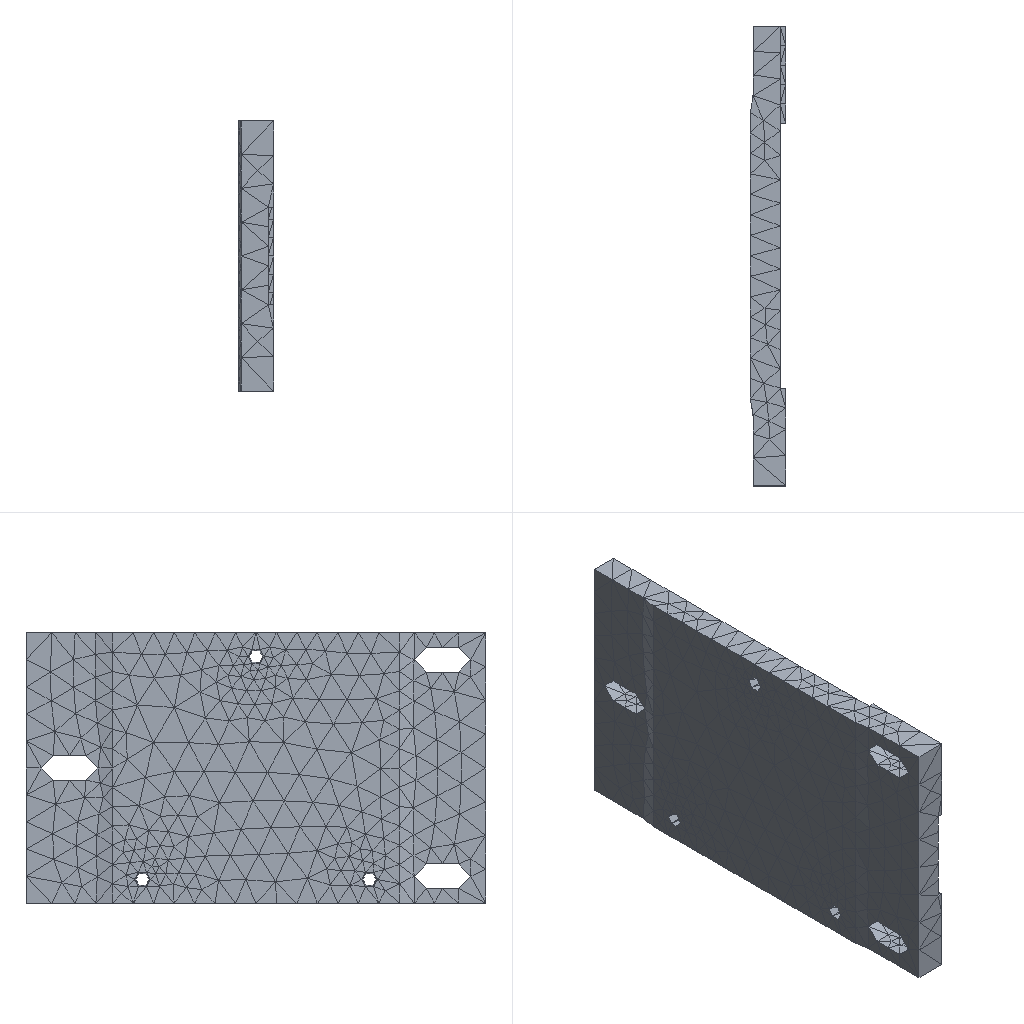Simulation study | nx simcenter
Set-up summary:
category,name,step,type,value,unit,region
solver,nx_nastran (Simcenter)
units,not stated in the deck,,not stated
analysis,deck,,static,static
analysis,solution,,SOL,101
load_step,SUBCASE 1,1,SUBCASE,SPC=1 LOAD=2
load_step,requested,,,1
mesh,nodes,,,5373
mesh,elements,,,2702
element_type,CTETRA,,solid,2702
load,nodal force total,,FX,750000.028,model units
load,nodal force total,,FY,0.0,model units
load,nodal force total,,FZ,0.0,model units
load,load commands in deck,,count,625
bc,support commands in deck,,count,345
analysis,NX solution 0,,Structural,Linear Statics - Single Constraint
check,setup vs results,,match,every grid point's frame and coordinates and every element id; grid points of CTETRA elements
Nastran input file, long lists of numbers shortened:
$*$$$$$$$$$$$$$$$$$$$$$$$$$$$$$$$$$$$$$$$$$$$$$$$$$$$$$$$$$$$$$$$$$
$*
$*                    NX v10.0.0.24 TRANSLATOR
$*                    FOR NX NASTRAN VERSION 10.0
$ (33 more lines like these left out)
ASSIGN OUTPUT2='153_sim1-solution_1.op2' UNIT=12
$*
$*$$$$$$$$$$$$$$$$$$$$$$$$$$$$$$$$$$$
$*
$* EXECUTIVE CONTROL
$*
$*$$$$$$$$$$$$$$$$$$$$$$$$$$$$$$$$$$$
$*
ID,NASTRAN,153_sim1-solution_1
SOL 101
CEND
$*
$*$$$$$$$$$$$$$$$$$$$$$$$$$$$$$$$$$$$
$*
$* CASE CONTROL
$*
$*$$$$$$$$$$$$$$$$$$$$$$$$$$$$$$$$$$$
$*
TITLE = Solution 1
ECHO = NONE
SPC = 1
OUTPUT
BCRESULTS(TRACTION,FORCE,PLOT) = ALL
DISPLACEMENT(PLOT) = ALL
ESE(PLOT) = ALL
FORCE(PLOT,CORNER) = ALL
OLOAD(PLOT) = ALL
SPCFORCES(PLOT) = ALL
STRAIN(PLOT,FIBER,CORNER) = ALL
STRESS(PLOT,CORNER) = ALL
$*  NX Step: Subcase - Static Loads 1
SUBCASE 1
LABEL = Subcase - Static Loads 1
LOAD = 2
$*
$*$$$$$$$$$$$$$$$$$$$$$$$$$$$$$$$$$$$
$*
$* BULK DATA
$*
$*$$$$$$$$$$$$$$$$$$$$$$$$$$$$$$$$$$$
$*
BEGIN BULK
$*
$* PARAM CARDS
$*
PARAM      K6ROT100.0000
PARAM     OIBULK     YES
PARAM    OMACHPR     YES
PARAM       POST      -2
PARAM    POSTEXT     YES
PARAM    UNITSYS   MN-MM
$*
$* GRID CARDS
$*
GRID*               5312               05.2113121033E+01-3.999267883E+02+
*       4.6302730560E+01               0
GRID*               5313               05.2113121033E+01-3.999267883E+02+
*       -3.697266102E+00               0
$ (10742 more lines like these left out)
$*
$* ELEMENT CARDS
$*
$*  NX Mesh Collector: Solid(1)
$*  NX Mesh: 3d_mesh(1)
CTETRA         1       1    4979       1    4978    2647      90      91+
+           4983    3203      92    3202
CTETRA         2       1       2    2594       3    2590      93      94+
+             95      96    2999      97
$ (5400 more lines like these left out)
$*
$* PROPERTY CARDS
$*
$*  NX Property: PSOLID1
PSOLID         1       1       0                           SMECH
$*
$* MATERIAL CARDS
$*
$*  NX Material: 2A12
MAT1           17.3119+7        0.3300002.8000-62.1355-5
MATT1          1       1               2               3
TABLEM1        1                                                        +
+        20.00007.3119+7 21.11007.3119+7 23.89007.3119+7 37.78007.3119+7+
+        51.67007.3119+7 65.56007.2429+7 79.44007.2429+7 93.33007.1739+7+
+       107.22007.1049+7121.11007.0359+7135.00006.9670+7148.89006.8980+7+
+       162.78006.8290+7176.67006.6910+7190.56006.6221+7204.44006.4841+7+
+       218.33006.3461+7232.22006.1392+7246.11006.0012+7260.00005.8633+7+
+       273.89005.7253+7287.78005.5184+7301.67005.3804+7315.56005.1735+7+
+       329.44004.9665+7343.33004.7596+7357.22004.6216+7371.11004.4147+7+
+           ENDT
TABLEM1        2                                                        +
+        20.00000.330000 21.11000.330000    ENDT
TABLEM1        3                                                        +
+        20.00002.1600-5 93.33002.2500-5107.22002.2662-5121.11002.2824-5+
+       135.00002.2968-5148.89002.3130-5162.78002.3274-5176.67002.3418-5+
+       190.56002.3544-5204.44002.3688-5218.33002.3814-5232.22002.3958-5+
+       246.11002.4066-5260.00002.4192-5273.89002.4300-5287.78002.4408-5+
+       301.67002.4498-5315.56002.4606-5329.44002.4696-5343.33002.4786-5+
+       357.22002.4876-5371.11002.4984-5385.00002.5110-5398.89002.5254-5+
+       412.78002.5398-5426.67002.5560-5    ENDT
$*
$* LOAD AND CONSTRAINT CARDS
$*
$*  NX Load and Constraint: Fixed(1)
SPC            1    3488  123456  0.0000
SPC            1    3489  123456  0.0000
SPC            1    3490  123456  0.0000
SPC            1    3491  123456  0.0000
$ (341 more lines like these left out)
$*  NX Load and Constraint: Force(1)
FORCE          2    4121       0248.11261.000000  0.0000  0.0000
FORCE          2    4122       0378.38081.000000  0.0000  0.0000
FORCE          2    4123       0268.01981.000000  0.0000  0.0000
FORCE          2    4124       0389.56501.000000  0.0000  0.0000
$ (621 more lines like these left out)
ENDDATA 7fe41b5a
Results summary:
result,analysis,,,static
result,last_loadstep,,,1
result,primary field,,,displacements
result,reaction total,,FX,-750000.125,model units
result,reaction total,,FY,-0.03687,model units
result,reaction total,,FZ,0.006287,model units
result,NX solution 0,,loadcases,1,mm